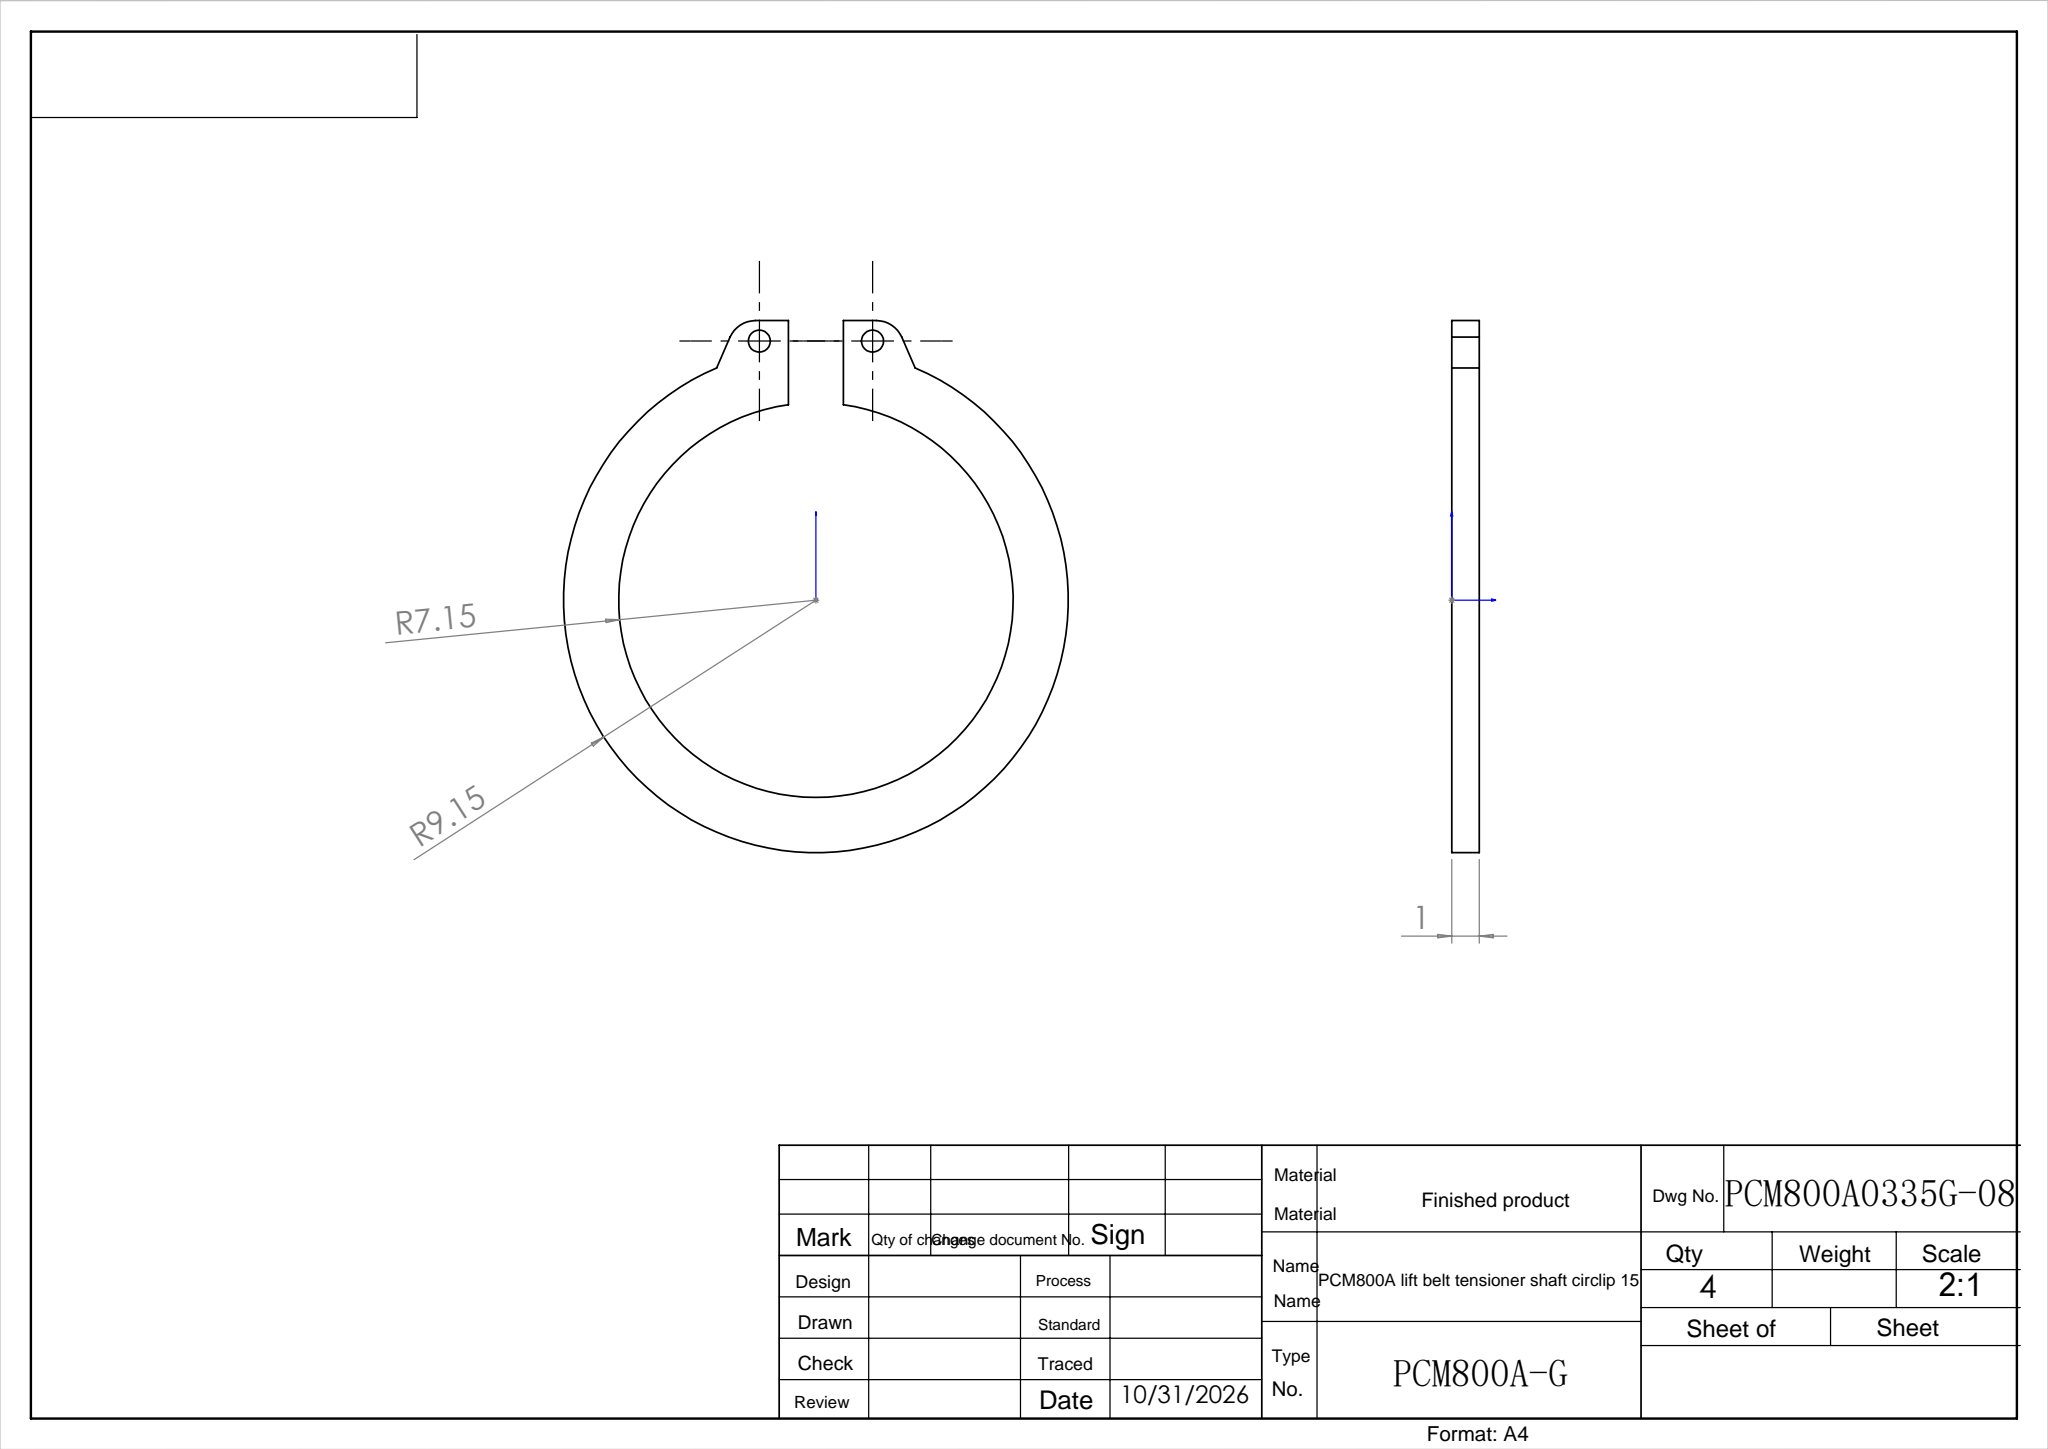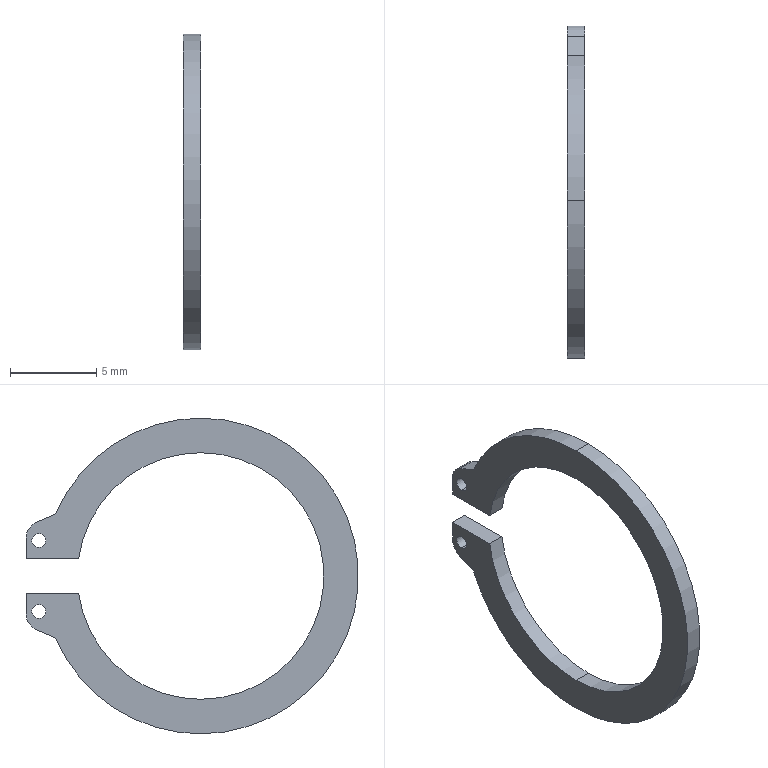Part | SolidWorks | features Boss 1, Cut 1, Extrusion 1 | 1 solid | 20 faces | box 1 x 19.276 x 18.3 mm | volume 102.745 mm3 | cylinder 12 | plane 8 | commonest cylinder face diameters 0.8 x4 14.3 x3 18.3 x3 2 x2
STEP:
#1=CARTESIAN_POINT('',(0.,9.383,-1.652));
#2=VERTEX_POINT('',#1);
#3=CARTESIAN_POINT('',(0.,9.383,-2.452));
#4=VERTEX_POINT('',#3);
#5=CARTESIAN_POINT('',(0.,9.383,-2.052));
#6=DIRECTION('',(1.,0.,0.));
#7=DIRECTION('',(0.,0.,1.));
#8=AXIS2_PLACEMENT_3D('',#5,#6,#7);
#9=CIRCLE('',#8,0.4);
#10=EDGE_CURVE('',#2,#4,#9,.T.);
#11=ORIENTED_EDGE('',*,*,#10,.F.);
#12=CARTESIAN_POINT('',(1.,9.383,-1.652));
#13=VERTEX_POINT('',#12);
#14=CARTESIAN_POINT('',(0.,9.383,-1.652));
#15=DIRECTION('',(1.,0.,0.));
#16=VECTOR('',#15,1000.);
#17=LINE('',#14,#16);
#18=EDGE_CURVE('',#2,#13,#17,.T.);
#19=ORIENTED_EDGE('',*,*,#18,.T.);
#20=CARTESIAN_POINT('',(1.,9.383,-2.452));
#21=VERTEX_POINT('',#20);
#22=CARTESIAN_POINT('',(1.,9.383,-2.052));
#23=DIRECTION('',(1.,0.,0.));
#24=DIRECTION('',(0.,0.,1.));
#25=AXIS2_PLACEMENT_3D('',#22,#23,#24);
#26=CIRCLE('',#25,0.4);
#27=EDGE_CURVE('',#13,#21,#26,.T.);
#28=ORIENTED_EDGE('',*,*,#27,.T.);
#29=CARTESIAN_POINT('',(0.,9.383,-2.452));
#30=DIRECTION('',(1.,0.,0.));
#31=VECTOR('',#30,1000.);
#32=LINE('',#29,#31);
#33=EDGE_CURVE('',#4,#21,#32,.T.);
#34=ORIENTED_EDGE('',*,*,#33,.F.);
#35=EDGE_LOOP('',(#11,#19,#28,#34));
#36=FACE_OUTER_BOUND('',#35,.T.);
#37=CARTESIAN_POINT('',(0.,9.383,-2.052));
#38=DIRECTION('',(1.,0.,0.));
#39=DIRECTION('',(0.,0.,-1.));
#40=AXIS2_PLACEMENT_3D('',#37,#38,#39);
#41=CYLINDRICAL_SURFACE('',#40,0.4);
#42=ADVANCED_FACE('',(#36),#41,.F.);
#43=CARTESIAN_POINT('',(0.,9.383,2.452));
#44=VERTEX_POINT('',#43);
#45=CARTESIAN_POINT('',(0.,9.383,1.652));
#46=VERTEX_POINT('',#45);
#47=CARTESIAN_POINT('',(0.,9.383,2.052));
#48=DIRECTION('',(1.,0.,0.));
#49=DIRECTION('',(0.,0.,-1.));
#50=AXIS2_PLACEMENT_3D('',#47,#48,#49);
#51=CIRCLE('',#50,0.4);
#52=EDGE_CURVE('',#44,#46,#51,.T.);
#53=ORIENTED_EDGE('',*,*,#52,.F.);
#54=CARTESIAN_POINT('',(1.,9.383,2.452));
#55=VERTEX_POINT('',#54);
#56=CARTESIAN_POINT('',(0.,9.383,2.452));
#57=DIRECTION('',(1.,0.,0.));
#58=VECTOR('',#57,1000.);
#59=LINE('',#56,#58);
#60=EDGE_CURVE('',#44,#55,#59,.T.);
#61=ORIENTED_EDGE('',*,*,#60,.T.);
#62=CARTESIAN_POINT('',(1.,9.383,1.652));
#63=VERTEX_POINT('',#62);
#64=CARTESIAN_POINT('',(1.,9.383,2.052));
#65=DIRECTION('',(1.,0.,0.));
#66=DIRECTION('',(0.,0.,-1.));
#67=AXIS2_PLACEMENT_3D('',#64,#65,#66);
#68=CIRCLE('',#67,0.4);
#69=EDGE_CURVE('',#55,#63,#68,.T.);
#70=ORIENTED_EDGE('',*,*,#69,.T.);
#71=CARTESIAN_POINT('',(0.,9.383,1.652));
#72=DIRECTION('',(1.,0.,0.));
#73=VECTOR('',#72,1000.);
#74=LINE('',#71,#73);
#75=EDGE_CURVE('',#46,#63,#74,.T.);
#76=ORIENTED_EDGE('',*,*,#75,.F.);
#77=EDGE_LOOP('',(#53,#61,#70,#76));
#78=FACE_OUTER_BOUND('',#77,.T.);
#79=CARTESIAN_POINT('',(0.,9.383,2.052));
#80=DIRECTION('',(1.,0.,0.));
#81=DIRECTION('',(0.,0.,-1.));
#82=AXIS2_PLACEMENT_3D('',#79,#80,#81);
#83=CYLINDRICAL_SURFACE('',#82,0.4);
#84=ADVANCED_FACE('',(#78),#83,.F.);
#85=CARTESIAN_POINT('',(1.,0.,7.15));
#86=VERTEX_POINT('',#85);
#87=CARTESIAN_POINT('',(1.,0.,-7.15));
#88=VERTEX_POINT('',#87);
#89=CARTESIAN_POINT('',(1.,0.,0.));
#90=DIRECTION('',(1.,0.,0.));
#91=DIRECTION('',(0.,0.,-1.));
#92=AXIS2_PLACEMENT_3D('',#89,#90,#91);
#93=CIRCLE('',#92,7.15);
#94=EDGE_CURVE('',#86,#88,#93,.T.);
#95=ORIENTED_EDGE('',*,*,#94,.T.);
#96=CARTESIAN_POINT('',(0.,0.,-7.15));
#97=VERTEX_POINT('',#96);
#98=CARTESIAN_POINT('',(1.,0.,-7.15));
#99=DIRECTION('',(-1.,0.,0.));
#100=VECTOR('',#99,1000.);
#101=LINE('',#98,#100);
#102=EDGE_CURVE('',#88,#97,#101,.T.);
#103=ORIENTED_EDGE('',*,*,#102,.T.);
#104=CARTESIAN_POINT('',(0.,0.,7.15));
#105=VERTEX_POINT('',#104);
#106=CARTESIAN_POINT('',(0.,0.,0.));
#107=DIRECTION('',(1.,0.,0.));
#108=DIRECTION('',(0.,0.,-1.));
#109=AXIS2_PLACEMENT_3D('',#106,#107,#108);
#110=CIRCLE('',#109,7.15);
#111=EDGE_CURVE('',#105,#97,#110,.T.);
#112=ORIENTED_EDGE('',*,*,#111,.F.);
#113=CARTESIAN_POINT('',(1.,0.,7.15));
#114=DIRECTION('',(-1.,0.,0.));
#115=VECTOR('',#114,1000.);
#116=LINE('',#113,#115);
#117=EDGE_CURVE('',#86,#105,#116,.T.);
#118=ORIENTED_EDGE('',*,*,#117,.F.);
#119=EDGE_LOOP('',(#95,#103,#112,#118));
#120=FACE_OUTER_BOUND('',#119,.T.);
#121=CARTESIAN_POINT('',(1.,0.,0.));
#122=DIRECTION('',(-1.,0.,0.));
#123=DIRECTION('',(0.,0.,1.));
#124=AXIS2_PLACEMENT_3D('',#121,#122,#123);
#125=CYLINDRICAL_SURFACE('',#124,7.15);
#126=ADVANCED_FACE('',(#120),#125,.F.);
#127=CARTESIAN_POINT('',(1.,7.08,1.));
#128=VERTEX_POINT('',#127);
#129=CARTESIAN_POINT('',(1.,0.,0.));
#130=DIRECTION('',(1.,0.,0.));
#131=DIRECTION('',(0.,0.,-1.));
#132=AXIS2_PLACEMENT_3D('',#129,#130,#131);
#133=CIRCLE('',#132,7.15);
#134=EDGE_CURVE('',#128,#86,#133,.T.);
#135=ORIENTED_EDGE('',*,*,#134,.T.);
#136=ORIENTED_EDGE('',*,*,#117,.T.);
#137=CARTESIAN_POINT('',(0.,7.08,1.));
#138=VERTEX_POINT('',#137);
#139=CARTESIAN_POINT('',(0.,0.,0.));
#140=DIRECTION('',(1.,0.,0.));
#141=DIRECTION('',(0.,0.,-1.));
#142=AXIS2_PLACEMENT_3D('',#139,#140,#141);
#143=CIRCLE('',#142,7.15);
#144=EDGE_CURVE('',#138,#105,#143,.T.);
#145=ORIENTED_EDGE('',*,*,#144,.F.);
#146=CARTESIAN_POINT('',(1.,7.08,1.));
#147=DIRECTION('',(-1.,0.,0.));
#148=VECTOR('',#147,1000.);
#149=LINE('',#146,#148);
#150=EDGE_CURVE('',#128,#138,#149,.T.);
#151=ORIENTED_EDGE('',*,*,#150,.F.);
#152=EDGE_LOOP('',(#135,#136,#145,#151));
#153=FACE_OUTER_BOUND('',#152,.T.);
#154=CARTESIAN_POINT('',(1.,0.,0.));
#155=DIRECTION('',(-1.,0.,0.));
#156=DIRECTION('',(0.,0.,1.));
#157=AXIS2_PLACEMENT_3D('',#154,#155,#156);
#158=CYLINDRICAL_SURFACE('',#157,7.15);
#159=ADVANCED_FACE('',(#153),#158,.F.);
#160=CARTESIAN_POINT('',(1.,0.,-9.15));
#161=VERTEX_POINT('',#160);
#162=CARTESIAN_POINT('',(1.,8.412,-3.6));
#163=VERTEX_POINT('',#162);
#164=CARTESIAN_POINT('',(1.,0.,0.));
#165=DIRECTION('',(1.,0.,0.));
#166=DIRECTION('',(0.,0.,-1.));
#167=AXIS2_PLACEMENT_3D('',#164,#165,#166);
#168=CIRCLE('',#167,9.15);
#169=EDGE_CURVE('',#161,#163,#168,.T.);
#170=ORIENTED_EDGE('',*,*,#169,.F.);
#171=CARTESIAN_POINT('',(0.,0.,-9.15));
#172=VERTEX_POINT('',#171);
#173=CARTESIAN_POINT('',(1.,0.,-9.15));
#174=DIRECTION('',(-1.,0.,0.));
#175=VECTOR('',#174,1000.);
#176=LINE('',#173,#175);
#177=EDGE_CURVE('',#161,#172,#176,.T.);
#178=ORIENTED_EDGE('',*,*,#177,.T.);
#179=CARTESIAN_POINT('',(0.,8.412,-3.6));
#180=VERTEX_POINT('',#179);
#181=CARTESIAN_POINT('',(0.,0.,0.));
#182=DIRECTION('',(1.,0.,0.));
#183=DIRECTION('',(0.,0.,-1.));
#184=AXIS2_PLACEMENT_3D('',#181,#182,#183);
#185=CIRCLE('',#184,9.15);
#186=EDGE_CURVE('',#172,#180,#185,.T.);
#187=ORIENTED_EDGE('',*,*,#186,.T.);
#188=CARTESIAN_POINT('',(0.,8.412,-3.6));
#189=DIRECTION('',(1.,0.,0.));
#190=VECTOR('',#189,1000.);
#191=LINE('',#188,#190);
#192=EDGE_CURVE('',#180,#163,#191,.T.);
#193=ORIENTED_EDGE('',*,*,#192,.T.);
#194=EDGE_LOOP('',(#170,#178,#187,#193));
#195=FACE_OUTER_BOUND('',#194,.T.);
#196=CARTESIAN_POINT('',(1.,0.,0.));
#197=DIRECTION('',(-1.,0.,0.));
#198=DIRECTION('',(0.,0.,1.));
#199=AXIS2_PLACEMENT_3D('',#196,#197,#198);
#200=CYLINDRICAL_SURFACE('',#199,9.15);
#201=ADVANCED_FACE('',(#195),#200,.T.);
#202=ORIENTED_EDGE('',*,*,#177,.F.);
#203=CARTESIAN_POINT('',(1.,0.,9.15));
#204=VERTEX_POINT('',#203);
#205=CARTESIAN_POINT('',(1.,0.,0.));
#206=DIRECTION('',(1.,0.,0.));
#207=DIRECTION('',(0.,0.,-1.));
#208=AXIS2_PLACEMENT_3D('',#205,#206,#207);
#209=CIRCLE('',#208,9.15);
#210=EDGE_CURVE('',#204,#161,#209,.T.);
#211=ORIENTED_EDGE('',*,*,#210,.F.);
#212=CARTESIAN_POINT('',(0.,0.,9.15));
#213=VERTEX_POINT('',#212);
#214=CARTESIAN_POINT('',(1.,0.,9.15));
#215=DIRECTION('',(-1.,0.,0.));
#216=VECTOR('',#215,1000.);
#217=LINE('',#214,#216);
#218=EDGE_CURVE('',#204,#213,#217,.T.);
#219=ORIENTED_EDGE('',*,*,#218,.T.);
#220=CARTESIAN_POINT('',(0.,0.,0.));
#221=DIRECTION('',(1.,0.,0.));
#222=DIRECTION('',(0.,0.,-1.));
#223=AXIS2_PLACEMENT_3D('',#220,#221,#222);
#224=CIRCLE('',#223,9.15);
#225=EDGE_CURVE('',#213,#172,#224,.T.);
#226=ORIENTED_EDGE('',*,*,#225,.T.);
#227=EDGE_LOOP('',(#202,#211,#219,#226));
#228=FACE_OUTER_BOUND('',#227,.T.);
#229=CARTESIAN_POINT('',(1.,0.,0.));
#230=DIRECTION('',(-1.,0.,0.));
#231=DIRECTION('',(0.,0.,1.));
#232=AXIS2_PLACEMENT_3D('',#229,#230,#231);
#233=CYLINDRICAL_SURFACE('',#232,9.15);
#234=ADVANCED_FACE('',(#228),#233,.T.);
#235=CARTESIAN_POINT('',(1.,10.126,1.));
#236=VERTEX_POINT('',#235);
#237=CARTESIAN_POINT('',(1.,0.,1.));
#238=DIRECTION('',(0.,-1.,0.));
#239=VECTOR('',#238,1000.);
#240=LINE('',#237,#239);
#241=EDGE_CURVE('',#236,#128,#240,.T.);
#242=ORIENTED_EDGE('',*,*,#241,.F.);
#243=CARTESIAN_POINT('',(1.,10.126,2.197));
#244=VERTEX_POINT('',#243);
#245=CARTESIAN_POINT('',(1.,10.126,1.));
#246=DIRECTION('',(0.,0.000003702,1.));
#247=VECTOR('',#246,1000.);
#248=LINE('',#245,#247);
#249=EDGE_CURVE('',#236,#244,#248,.T.);
#250=ORIENTED_EDGE('',*,*,#249,.T.);
#251=CARTESIAN_POINT('',(1.,9.526,3.113));
#252=VERTEX_POINT('',#251);
#253=CARTESIAN_POINT('',(1.,9.126,2.197));
#254=DIRECTION('',(1.,0.,0.));
#255=DIRECTION('',(0.,0.,1.));
#256=AXIS2_PLACEMENT_3D('',#253,#254,#255);
#257=CIRCLE('',#256,1.);
#258=EDGE_CURVE('',#244,#252,#257,.T.);
#259=ORIENTED_EDGE('',*,*,#258,.T.);
#260=CARTESIAN_POINT('',(1.,8.412,3.6));
#261=VERTEX_POINT('',#260);
#262=CARTESIAN_POINT('',(1.,9.526,3.113));
#263=DIRECTION('',(0.,-0.9164,0.4002));
#264=VECTOR('',#263,1000.);
#265=LINE('',#262,#264);
#266=EDGE_CURVE('',#252,#261,#265,.T.);
#267=ORIENTED_EDGE('',*,*,#266,.T.);
#268=CARTESIAN_POINT('',(1.,0.,0.));
#269=DIRECTION('',(1.,0.,0.));
#270=DIRECTION('',(0.,0.,-1.));
#271=AXIS2_PLACEMENT_3D('',#268,#269,#270);
#272=CIRCLE('',#271,9.15);
#273=EDGE_CURVE('',#261,#204,#272,.T.);
#274=ORIENTED_EDGE('',*,*,#273,.T.);
#275=ORIENTED_EDGE('',*,*,#210,.T.);
#276=ORIENTED_EDGE('',*,*,#169,.T.);
#277=CARTESIAN_POINT('',(1.,9.526,-3.113));
#278=VERTEX_POINT('',#277);
#279=CARTESIAN_POINT('',(1.,9.526,-3.113));
#280=DIRECTION('',(0.,0.9164,0.4002));
#281=VECTOR('',#280,1000.);
#282=LINE('',#279,#281);
#283=EDGE_CURVE('',#163,#278,#282,.T.);
#284=ORIENTED_EDGE('',*,*,#283,.T.);
#285=CARTESIAN_POINT('',(1.,10.126,-2.197));
#286=VERTEX_POINT('',#285);
#287=CARTESIAN_POINT('',(1.,9.126,-2.197));
#288=DIRECTION('',(1.,0.,0.));
#289=DIRECTION('',(0.,0.,-1.));
#290=AXIS2_PLACEMENT_3D('',#287,#288,#289);
#291=CIRCLE('',#290,1.);
#292=EDGE_CURVE('',#278,#286,#291,.T.);
#293=ORIENTED_EDGE('',*,*,#292,.T.);
#294=CARTESIAN_POINT('',(1.,10.126,-1.));
#295=VERTEX_POINT('',#294);
#296=CARTESIAN_POINT('',(1.,10.126,-1.));
#297=DIRECTION('',(0.,-0.000003702,1.));
#298=VECTOR('',#297,1000.);
#299=LINE('',#296,#298);
#300=EDGE_CURVE('',#286,#295,#299,.T.);
#301=ORIENTED_EDGE('',*,*,#300,.T.);
#302=CARTESIAN_POINT('',(1.,7.08,-1.));
#303=VERTEX_POINT('',#302);
#304=CARTESIAN_POINT('',(1.,0.,-1.));
#305=DIRECTION('',(0.,1.,0.));
#306=VECTOR('',#305,1000.);
#307=LINE('',#304,#306);
#308=EDGE_CURVE('',#303,#295,#307,.T.);
#309=ORIENTED_EDGE('',*,*,#308,.F.);
#310=CARTESIAN_POINT('',(1.,0.,0.));
#311=DIRECTION('',(1.,0.,0.));
#312=DIRECTION('',(0.,0.,-1.));
#313=AXIS2_PLACEMENT_3D('',#310,#311,#312);
#314=CIRCLE('',#313,7.15);
#315=EDGE_CURVE('',#88,#303,#314,.T.);
#316=ORIENTED_EDGE('',*,*,#315,.F.);
#317=ORIENTED_EDGE('',*,*,#94,.F.);
#318=ORIENTED_EDGE('',*,*,#134,.F.);
#319=EDGE_LOOP('',(#242,#250,#259,#267,#274,#275,#276,#284,#293,#301,#309,#316,#317,#318));
#320=FACE_OUTER_BOUND('',#319,.T.);
#321=CARTESIAN_POINT('',(1.,9.383,2.052));
#322=DIRECTION('',(1.,0.,0.));
#323=DIRECTION('',(0.,0.,-1.));
#324=AXIS2_PLACEMENT_3D('',#321,#322,#323);
#325=CIRCLE('',#324,0.4);
#326=EDGE_CURVE('',#63,#55,#325,.T.);
#327=ORIENTED_EDGE('',*,*,#326,.F.);
#328=ORIENTED_EDGE('',*,*,#69,.F.);
#329=EDGE_LOOP('',(#327,#328));
#330=FACE_BOUND('',#329,.T.);
#331=CARTESIAN_POINT('',(1.,9.383,-2.052));
#332=DIRECTION('',(1.,0.,0.));
#333=DIRECTION('',(0.,0.,1.));
#334=AXIS2_PLACEMENT_3D('',#331,#332,#333);
#335=CIRCLE('',#334,0.4);
#336=EDGE_CURVE('',#21,#13,#335,.T.);
#337=ORIENTED_EDGE('',*,*,#336,.F.);
#338=ORIENTED_EDGE('',*,*,#27,.F.);
#339=EDGE_LOOP('',(#337,#338));
#340=FACE_BOUND('',#339,.T.);
#341=CARTESIAN_POINT('',(1.,0.,0.));
#342=DIRECTION('',(1.,0.,0.));
#343=DIRECTION('',(0.,0.,-1.));
#344=AXIS2_PLACEMENT_3D('',#341,#342,#343);
#345=PLANE('',#344);
#346=ADVANCED_FACE('',(#320,#330,#340),#345,.T.);
#347=CARTESIAN_POINT('',(0.,8.412,3.6));
#348=VERTEX_POINT('',#347);
#349=CARTESIAN_POINT('',(0.,0.,0.));
#350=DIRECTION('',(1.,0.,0.));
#351=DIRECTION('',(0.,0.,-1.));
#352=AXIS2_PLACEMENT_3D('',#349,#350,#351);
#353=CIRCLE('',#352,9.15);
#354=EDGE_CURVE('',#348,#213,#353,.T.);
#355=ORIENTED_EDGE('',*,*,#354,.F.);
#356=CARTESIAN_POINT('',(0.,9.526,3.113));
#357=VERTEX_POINT('',#356);
#358=CARTESIAN_POINT('',(0.,9.526,3.113));
#359=DIRECTION('',(0.,-0.9164,0.4002));
#360=VECTOR('',#359,1000.);
#361=LINE('',#358,#360);
#362=EDGE_CURVE('',#357,#348,#361,.T.);
#363=ORIENTED_EDGE('',*,*,#362,.F.);
#364=CARTESIAN_POINT('',(0.,10.126,2.197));
#365=VERTEX_POINT('',#364);
#366=CARTESIAN_POINT('',(0.,9.126,2.197));
#367=DIRECTION('',(1.,0.,0.));
#368=DIRECTION('',(0.,0.,1.));
#369=AXIS2_PLACEMENT_3D('',#366,#367,#368);
#370=CIRCLE('',#369,1.);
#371=EDGE_CURVE('',#365,#357,#370,.T.);
#372=ORIENTED_EDGE('',*,*,#371,.F.);
#373=CARTESIAN_POINT('',(0.,10.126,1.));
#374=VERTEX_POINT('',#373);
#375=CARTESIAN_POINT('',(0.,10.126,1.));
#376=DIRECTION('',(0.,0.000003702,1.));
#377=VECTOR('',#376,1000.);
#378=LINE('',#375,#377);
#379=EDGE_CURVE('',#374,#365,#378,.T.);
#380=ORIENTED_EDGE('',*,*,#379,.F.);
#381=CARTESIAN_POINT('',(0.,0.,1.));
#382=DIRECTION('',(0.,-1.,0.));
#383=VECTOR('',#382,1000.);
#384=LINE('',#381,#383);
#385=EDGE_CURVE('',#374,#138,#384,.T.);
#386=ORIENTED_EDGE('',*,*,#385,.T.);
#387=ORIENTED_EDGE('',*,*,#144,.T.);
#388=ORIENTED_EDGE('',*,*,#111,.T.);
#389=CARTESIAN_POINT('',(0.,7.08,-1.));
#390=VERTEX_POINT('',#389);
#391=CARTESIAN_POINT('',(0.,0.,0.));
#392=DIRECTION('',(1.,0.,0.));
#393=DIRECTION('',(0.,0.,-1.));
#394=AXIS2_PLACEMENT_3D('',#391,#392,#393);
#395=CIRCLE('',#394,7.15);
#396=EDGE_CURVE('',#97,#390,#395,.T.);
#397=ORIENTED_EDGE('',*,*,#396,.T.);
#398=CARTESIAN_POINT('',(0.,10.126,-1.));
#399=VERTEX_POINT('',#398);
#400=CARTESIAN_POINT('',(0.,0.,-1.));
#401=DIRECTION('',(0.,1.,0.));
#402=VECTOR('',#401,1000.);
#403=LINE('',#400,#402);
#404=EDGE_CURVE('',#390,#399,#403,.T.);
#405=ORIENTED_EDGE('',*,*,#404,.T.);
#406=CARTESIAN_POINT('',(0.,10.126,-2.197));
#407=VERTEX_POINT('',#406);
#408=CARTESIAN_POINT('',(0.,10.126,-1.));
#409=DIRECTION('',(0.,-0.000003702,1.));
#410=VECTOR('',#409,1000.);
#411=LINE('',#408,#410);
#412=EDGE_CURVE('',#407,#399,#411,.T.);
#413=ORIENTED_EDGE('',*,*,#412,.F.);
#414=CARTESIAN_POINT('',(0.,9.526,-3.113));
#415=VERTEX_POINT('',#414);
#416=CARTESIAN_POINT('',(0.,9.126,-2.197));
#417=DIRECTION('',(1.,0.,0.));
#418=DIRECTION('',(0.,0.,-1.));
#419=AXIS2_PLACEMENT_3D('',#416,#417,#418);
#420=CIRCLE('',#419,1.);
#421=EDGE_CURVE('',#415,#407,#420,.T.);
#422=ORIENTED_EDGE('',*,*,#421,.F.);
#423=CARTESIAN_POINT('',(0.,9.526,-3.113));
#424=DIRECTION('',(0.,0.9164,0.4002));
#425=VECTOR('',#424,1000.);
#426=LINE('',#423,#425);
#427=EDGE_CURVE('',#180,#415,#426,.T.);
#428=ORIENTED_EDGE('',*,*,#427,.F.);
#429=ORIENTED_EDGE('',*,*,#186,.F.);
#430=ORIENTED_EDGE('',*,*,#225,.F.);
#431=EDGE_LOOP('',(#355,#363,#372,#380,#386,#387,#388,#397,#405,#413,#422,#428,#429,#430));
#432=FACE_OUTER_BOUND('',#431,.T.);
#433=CARTESIAN_POINT('',(0.,9.383,2.052));
#434=DIRECTION('',(1.,0.,0.));
#435=DIRECTION('',(0.,0.,-1.));
#436=AXIS2_PLACEMENT_3D('',#433,#434,#435);
#437=CIRCLE('',#436,0.4);
#438=EDGE_CURVE('',#46,#44,#437,.T.);
#439=ORIENTED_EDGE('',*,*,#438,.T.);
#440=ORIENTED_EDGE('',*,*,#52,.T.);
#441=EDGE_LOOP('',(#439,#440));
#442=FACE_BOUND('',#441,.T.);
#443=CARTESIAN_POINT('',(0.,9.383,-2.052));
#444=DIRECTION('',(1.,0.,0.));
#445=DIRECTION('',(0.,0.,1.));
#446=AXIS2_PLACEMENT_3D('',#443,#444,#445);
#447=CIRCLE('',#446,0.4);
#448=EDGE_CURVE('',#4,#2,#447,.T.);
#449=ORIENTED_EDGE('',*,*,#448,.T.);
#450=ORIENTED_EDGE('',*,*,#10,.T.);
#451=EDGE_LOOP('',(#449,#450));
#452=FACE_BOUND('',#451,.T.);
#453=CARTESIAN_POINT('',(0.,0.,0.));
#454=DIRECTION('',(1.,0.,0.));
#455=DIRECTION('',(0.,0.,-1.));
#456=AXIS2_PLACEMENT_3D('',#453,#454,#455);
#457=PLANE('',#456);
#458=ADVANCED_FACE('',(#432,#442,#452),#457,.F.);
#459=ORIENTED_EDGE('',*,*,#218,.F.);
#460=ORIENTED_EDGE('',*,*,#273,.F.);
#461=CARTESIAN_POINT('',(0.,8.412,3.6));
#462=DIRECTION('',(1.,0.,0.));
#463=VECTOR('',#462,1000.);
#464=LINE('',#461,#463);
#465=EDGE_CURVE('',#348,#261,#464,.T.);
#466=ORIENTED_EDGE('',*,*,#465,.F.);
#467=ORIENTED_EDGE('',*,*,#354,.T.);
#468=EDGE_LOOP('',(#459,#460,#466,#467));
#469=FACE_OUTER_BOUND('',#468,.T.);
#470=CARTESIAN_POINT('',(1.,0.,0.));
#471=DIRECTION('',(-1.,0.,0.));
#472=DIRECTION('',(0.,0.,1.));
#473=AXIS2_PLACEMENT_3D('',#470,#471,#472);
#474=CYLINDRICAL_SURFACE('',#473,9.15);
#475=ADVANCED_FACE('',(#469),#474,.T.);
#476=ORIENTED_EDGE('',*,*,#102,.F.);
#477=ORIENTED_EDGE('',*,*,#315,.T.);
#478=CARTESIAN_POINT('',(1.,7.08,-1.));
#479=DIRECTION('',(1.,0.,0.));
#480=VECTOR('',#479,1000.);
#481=LINE('',#478,#480);
#482=EDGE_CURVE('',#390,#303,#481,.T.);
#483=ORIENTED_EDGE('',*,*,#482,.F.);
#484=ORIENTED_EDGE('',*,*,#396,.F.);
#485=EDGE_LOOP('',(#476,#477,#483,#484));
#486=FACE_OUTER_BOUND('',#485,.T.);
#487=CARTESIAN_POINT('',(1.,0.,0.));
#488=DIRECTION('',(-1.,0.,0.));
#489=DIRECTION('',(0.,0.,1.));
#490=AXIS2_PLACEMENT_3D('',#487,#488,#489);
#491=CYLINDRICAL_SURFACE('',#490,7.15);
#492=ADVANCED_FACE('',(#486),#491,.F.);
#493=ORIENTED_EDGE('',*,*,#404,.F.);
#494=ORIENTED_EDGE('',*,*,#482,.T.);
#495=ORIENTED_EDGE('',*,*,#308,.T.);
#496=CARTESIAN_POINT('',(0.,10.126,-1.));
#497=DIRECTION('',(1.,0.,0.));
#498=VECTOR('',#497,1000.);
#499=LINE('',#496,#498);
#500=EDGE_CURVE('',#399,#295,#499,.T.);
#501=ORIENTED_EDGE('',*,*,#500,.F.);
#502=EDGE_LOOP('',(#493,#494,#495,#501));
#503=FACE_OUTER_BOUND('',#502,.T.);
#504=CARTESIAN_POINT('',(0.,0.,-1.));
#505=DIRECTION('',(0.,0.,-1.));
#506=DIRECTION('',(-1.,0.,0.));
#507=AXIS2_PLACEMENT_3D('',#504,#505,#506);
#508=PLANE('',#507);
#509=ADVANCED_FACE('',(#503),#508,.F.);
#510=ORIENTED_EDGE('',*,*,#241,.T.);
#511=ORIENTED_EDGE('',*,*,#150,.T.);
#512=ORIENTED_EDGE('',*,*,#385,.F.);
#513=CARTESIAN_POINT('',(0.,10.126,1.));
#514=DIRECTION('',(1.,0.,0.));
#515=VECTOR('',#514,1000.);
#516=LINE('',#513,#515);
#517=EDGE_CURVE('',#374,#236,#516,.T.);
#518=ORIENTED_EDGE('',*,*,#517,.T.);
#519=EDGE_LOOP('',(#510,#511,#512,#518));
#520=FACE_OUTER_BOUND('',#519,.T.);
#521=CARTESIAN_POINT('',(0.,0.,1.));
#522=DIRECTION('',(0.,0.,1.));
#523=DIRECTION('',(1.,0.,0.));
#524=AXIS2_PLACEMENT_3D('',#521,#522,#523);
#525=PLANE('',#524);
#526=ADVANCED_FACE('',(#520),#525,.F.);
#527=ORIENTED_EDGE('',*,*,#266,.F.);
#528=CARTESIAN_POINT('',(0.,9.526,3.113));
#529=DIRECTION('',(1.,0.,0.));
#530=VECTOR('',#529,1000.);
#531=LINE('',#528,#530);
#532=EDGE_CURVE('',#357,#252,#531,.T.);
#533=ORIENTED_EDGE('',*,*,#532,.F.);
#534=ORIENTED_EDGE('',*,*,#362,.T.);
#535=ORIENTED_EDGE('',*,*,#465,.T.);
#536=EDGE_LOOP('',(#527,#533,#534,#535));
#537=FACE_OUTER_BOUND('',#536,.T.);
#538=CARTESIAN_POINT('',(0.,9.526,3.113));
#539=DIRECTION('',(0.,0.4002,0.9164));
#540=DIRECTION('',(0.,-0.9164,0.4002));
#541=AXIS2_PLACEMENT_3D('',#538,#539,#540);
#542=PLANE('',#541);
#543=ADVANCED_FACE('',(#537),#542,.T.);
#544=ORIENTED_EDGE('',*,*,#258,.F.);
#545=CARTESIAN_POINT('',(0.,10.126,2.197));
#546=DIRECTION('',(1.,0.,0.));
#547=VECTOR('',#546,1000.);
#548=LINE('',#545,#547);
#549=EDGE_CURVE('',#365,#244,#548,.T.);
#550=ORIENTED_EDGE('',*,*,#549,.F.);
#551=ORIENTED_EDGE('',*,*,#371,.T.);
#552=ORIENTED_EDGE('',*,*,#532,.T.);
#553=EDGE_LOOP('',(#544,#550,#551,#552));
#554=FACE_OUTER_BOUND('',#553,.T.);
#555=CARTESIAN_POINT('',(0.,9.126,2.197));
#556=DIRECTION('',(1.,0.,0.));
#557=DIRECTION('',(0.,0.,-1.));
#558=AXIS2_PLACEMENT_3D('',#555,#556,#557);
#559=CYLINDRICAL_SURFACE('',#558,1.);
#560=ADVANCED_FACE('',(#554),#559,.T.);
#561=ORIENTED_EDGE('',*,*,#249,.F.);
#562=ORIENTED_EDGE('',*,*,#517,.F.);
#563=ORIENTED_EDGE('',*,*,#379,.T.);
#564=ORIENTED_EDGE('',*,*,#549,.T.);
#565=EDGE_LOOP('',(#561,#562,#563,#564));
#566=FACE_OUTER_BOUND('',#565,.T.);
#567=CARTESIAN_POINT('',(0.,10.126,1.));
#568=DIRECTION('',(0.,1.,-0.000003702));
#569=DIRECTION('',(0.,0.000003702,1.));
#570=AXIS2_PLACEMENT_3D('',#567,#568,#569);
#571=PLANE('',#570);
#572=ADVANCED_FACE('',(#566),#571,.T.);
#573=ORIENTED_EDGE('',*,*,#60,.F.);
#574=ORIENTED_EDGE('',*,*,#438,.F.);
#575=ORIENTED_EDGE('',*,*,#75,.T.);
#576=ORIENTED_EDGE('',*,*,#326,.T.);
#577=EDGE_LOOP('',(#573,#574,#575,#576));
#578=FACE_OUTER_BOUND('',#577,.T.);
#579=CARTESIAN_POINT('',(0.,9.383,2.052));
#580=DIRECTION('',(1.,0.,0.));
#581=DIRECTION('',(0.,0.,-1.));
#582=AXIS2_PLACEMENT_3D('',#579,#580,#581);
#583=CYLINDRICAL_SURFACE('',#582,0.4);
#584=ADVANCED_FACE('',(#578),#583,.F.);
#585=ORIENTED_EDGE('',*,*,#300,.F.);
#586=CARTESIAN_POINT('',(0.,10.126,-2.197));
#587=DIRECTION('',(1.,0.,0.));
#588=VECTOR('',#587,1000.);
#589=LINE('',#586,#588);
#590=EDGE_CURVE('',#407,#286,#589,.T.);
#591=ORIENTED_EDGE('',*,*,#590,.F.);
#592=ORIENTED_EDGE('',*,*,#412,.T.);
#593=ORIENTED_EDGE('',*,*,#500,.T.);
#594=EDGE_LOOP('',(#585,#591,#592,#593));
#595=FACE_OUTER_BOUND('',#594,.T.);
#596=CARTESIAN_POINT('',(0.,10.126,-1.));
#597=DIRECTION('',(0.,1.,0.000003702));
#598=DIRECTION('',(0.,-0.000003702,1.));
#599=AXIS2_PLACEMENT_3D('',#596,#597,#598);
#600=PLANE('',#599);
#601=ADVANCED_FACE('',(#595),#600,.T.);
#602=ORIENTED_EDGE('',*,*,#292,.F.);
#603=CARTESIAN_POINT('',(0.,9.526,-3.113));
#604=DIRECTION('',(1.,0.,0.));
#605=VECTOR('',#604,1000.);
#606=LINE('',#603,#605);
#607=EDGE_CURVE('',#415,#278,#606,.T.);
#608=ORIENTED_EDGE('',*,*,#607,.F.);
#609=ORIENTED_EDGE('',*,*,#421,.T.);
#610=ORIENTED_EDGE('',*,*,#590,.T.);
#611=EDGE_LOOP('',(#602,#608,#609,#610));
#612=FACE_OUTER_BOUND('',#611,.T.);
#613=CARTESIAN_POINT('',(0.,9.126,-2.197));
#614=DIRECTION('',(1.,0.,0.));
#615=DIRECTION('',(0.,0.,-1.));
#616=AXIS2_PLACEMENT_3D('',#613,#614,#615);
#617=CYLINDRICAL_SURFACE('',#616,1.);
#618=ADVANCED_FACE('',(#612),#617,.T.);
#619=ORIENTED_EDGE('',*,*,#283,.F.);
#620=ORIENTED_EDGE('',*,*,#192,.F.);
#621=ORIENTED_EDGE('',*,*,#427,.T.);
#622=ORIENTED_EDGE('',*,*,#607,.T.);
#623=EDGE_LOOP('',(#619,#620,#621,#622));
#624=FACE_OUTER_BOUND('',#623,.T.);
#625=CARTESIAN_POINT('',(0.,9.526,-3.113));
#626=DIRECTION('',(0.,0.4002,-0.9164));
#627=DIRECTION('',(0.,0.9164,0.4002));
#628=AXIS2_PLACEMENT_3D('',#625,#626,#627);
#629=PLANE('',#628);
#630=ADVANCED_FACE('',(#624),#629,.T.);
#631=ORIENTED_EDGE('',*,*,#18,.F.);
#632=ORIENTED_EDGE('',*,*,#448,.F.);
#633=ORIENTED_EDGE('',*,*,#33,.T.);
#634=ORIENTED_EDGE('',*,*,#336,.T.);
#635=EDGE_LOOP('',(#631,#632,#633,#634));
#636=FACE_OUTER_BOUND('',#635,.T.);
#637=CARTESIAN_POINT('',(0.,9.383,-2.052));
#638=DIRECTION('',(1.,0.,0.));
#639=DIRECTION('',(0.,0.,-1.));
#640=AXIS2_PLACEMENT_3D('',#637,#638,#639);
#641=CYLINDRICAL_SURFACE('',#640,0.4);
#642=ADVANCED_FACE('',(#636),#641,.F.);
#643=CLOSED_SHELL('',(#42,#84,#126,#159,#201,#234,#346,#458,#475,#492,#509,#526,#543,#560,#572,#584,#601,#618,#630,#642));
#644=MANIFOLD_SOLID_BREP('',#643);
#645=CARTESIAN_POINT('',(0.,0.,0.));
#646=DIRECTION('',(0.,0.,1.));
#647=DIRECTION('',(1.,0.,0.));
#648=AXIS2_PLACEMENT_3D('',#645,#646,#647);
#649=(LENGTH_UNIT()NAMED_UNIT(*)SI_UNIT(.MILLI.,.METRE.));
#650=UNCERTAINTY_MEASURE_WITH_UNIT(LENGTH_MEASURE(0.00001),#649,'','');
#651=(NAMED_UNIT(*)PLANE_ANGLE_UNIT()SI_UNIT($,.RADIAN.));
#652=(NAMED_UNIT(*)SI_UNIT($,.STERADIAN.)SOLID_ANGLE_UNIT());
#653=(GEOMETRIC_REPRESENTATION_CONTEXT(3)GLOBAL_UNCERTAINTY_ASSIGNED_CONTEXT((#650))GLOBAL_UNIT_ASSIGNED_CONTEXT((#649,#651,#652))REPRESENTATION_CONTEXT('',''));
#654=ADVANCED_BREP_SHAPE_REPRESENTATION('',(#644,#648),#653);